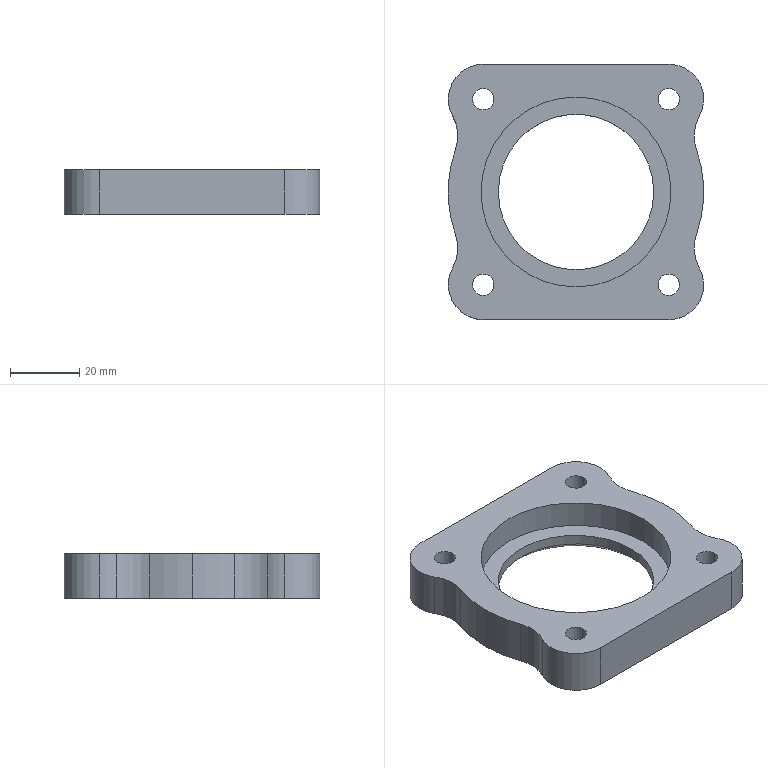Part | SolidWorks | features ICE 2, 3DProfileFeature 1, Chamfer 1, Extrusion 1, HoleWzd 1 | 1 solid | 34 faces | box 74 x 74 x 13 mm | volume 39480 mm3 | cylinder 27 | plane 5 | cone 2 | commonest cylinder face diameters 6.2 x8 20.2 x6 24 x6 74 x3 45 x2 55 x2
STEP:
#1=CARTESIAN_POINT('',(22.5,0.,2.));
#2=VERTEX_POINT('',#1);
#3=CARTESIAN_POINT('',(-22.5,0.,2.));
#4=VERTEX_POINT('',#3);
#5=CARTESIAN_POINT('',(0.,0.,2.));
#6=DIRECTION('',(0.,0.,-1.));
#7=DIRECTION('',(1.,0.,0.));
#8=AXIS2_PLACEMENT_3D('',#5,#6,#7);
#9=CIRCLE('',#8,22.5);
#10=EDGE_CURVE('',#2,#4,#9,.T.);
#11=ORIENTED_EDGE('',*,*,#10,.F.);
#12=CARTESIAN_POINT('',(24.5,0.,0.));
#13=VERTEX_POINT('',#12);
#14=CARTESIAN_POINT('',(22.5,0.,2.));
#15=DIRECTION('',(0.7071,0.,-0.7071));
#16=VECTOR('',#15,1000.);
#17=LINE('',#14,#16);
#18=EDGE_CURVE('',#2,#13,#17,.T.);
#19=ORIENTED_EDGE('',*,*,#18,.T.);
#20=CARTESIAN_POINT('',(-24.5,0.,0.));
#21=VERTEX_POINT('',#20);
#22=CARTESIAN_POINT('',(0.,0.,0.));
#23=DIRECTION('',(0.,0.,1.));
#24=DIRECTION('',(1.,0.,0.));
#25=AXIS2_PLACEMENT_3D('',#22,#23,#24);
#26=CIRCLE('',#25,24.5);
#27=EDGE_CURVE('',#21,#13,#26,.T.);
#28=ORIENTED_EDGE('',*,*,#27,.F.);
#29=CARTESIAN_POINT('',(-22.5,0.,2.));
#30=DIRECTION('',(-0.7071,0.,-0.7071));
#31=VECTOR('',#30,1000.);
#32=LINE('',#29,#31);
#33=EDGE_CURVE('',#4,#21,#32,.T.);
#34=ORIENTED_EDGE('',*,*,#33,.F.);
#35=EDGE_LOOP('',(#11,#19,#28,#34));
#36=FACE_OUTER_BOUND('',#35,.T.);
#37=CARTESIAN_POINT('',(0.,0.,2.));
#38=DIRECTION('',(0.,0.,-1.));
#39=DIRECTION('',(-1.,0.,0.));
#40=AXIS2_PLACEMENT_3D('',#37,#38,#39);
#41=CONICAL_SURFACE('',#40,22.5,0.7854);
#42=ADVANCED_FACE('',(#36),#41,.F.);
#43=ORIENTED_EDGE('',*,*,#10,.T.);
#44=CARTESIAN_POINT('',(-22.5,0.,5.));
#45=VERTEX_POINT('',#44);
#46=CARTESIAN_POINT('',(-22.5,0.,-0.001));
#47=DIRECTION('',(0.,0.,1.));
#48=VECTOR('',#47,1000.);
#49=LINE('',#46,#48);
#50=EDGE_CURVE('',#4,#45,#49,.T.);
#51=ORIENTED_EDGE('',*,*,#50,.T.);
#52=CARTESIAN_POINT('',(22.5,0.,5.));
#53=VERTEX_POINT('',#52);
#54=CARTESIAN_POINT('',(0.,0.,5.));
#55=DIRECTION('',(0.,0.,1.));
#56=DIRECTION('',(1.,0.,0.));
#57=AXIS2_PLACEMENT_3D('',#54,#55,#56);
#58=CIRCLE('',#57,22.5);
#59=EDGE_CURVE('',#45,#53,#58,.T.);
#60=ORIENTED_EDGE('',*,*,#59,.T.);
#61=CARTESIAN_POINT('',(22.5,0.,-0.001));
#62=DIRECTION('',(0.,0.,1.));
#63=VECTOR('',#62,1000.);
#64=LINE('',#61,#63);
#65=EDGE_CURVE('',#2,#53,#64,.T.);
#66=ORIENTED_EDGE('',*,*,#65,.F.);
#67=EDGE_LOOP('',(#43,#51,#60,#66));
#68=FACE_OUTER_BOUND('',#67,.T.);
#69=CARTESIAN_POINT('',(0.,0.,-0.001));
#70=DIRECTION('',(0.,0.,1.));
#71=DIRECTION('',(1.,0.,0.));
#72=AXIS2_PLACEMENT_3D('',#69,#70,#71);
#73=CYLINDRICAL_SURFACE('',#72,22.5);
#74=ADVANCED_FACE('',(#68),#73,.F.);
#75=CARTESIAN_POINT('',(-27.5,0.,5.));
#76=VERTEX_POINT('',#75);
#77=CARTESIAN_POINT('',(27.5,0.,5.));
#78=VERTEX_POINT('',#77);
#79=CARTESIAN_POINT('',(0.,0.,5.));
#80=DIRECTION('',(0.,0.,1.));
#81=DIRECTION('',(1.,0.,0.));
#82=AXIS2_PLACEMENT_3D('',#79,#80,#81);
#83=CIRCLE('',#82,27.5);
#84=EDGE_CURVE('',#76,#78,#83,.T.);
#85=ORIENTED_EDGE('',*,*,#84,.F.);
#86=CARTESIAN_POINT('',(-27.5,0.,13.));
#87=VERTEX_POINT('',#86);
#88=CARTESIAN_POINT('',(-27.5,0.,5.));
#89=DIRECTION('',(0.,0.,1.));
#90=VECTOR('',#89,1000.);
#91=LINE('',#88,#90);
#92=EDGE_CURVE('',#76,#87,#91,.T.);
#93=ORIENTED_EDGE('',*,*,#92,.T.);
#94=CARTESIAN_POINT('',(27.5,0.,13.));
#95=VERTEX_POINT('',#94);
#96=CARTESIAN_POINT('',(0.,0.,13.));
#97=DIRECTION('',(0.,0.,1.));
#98=DIRECTION('',(1.,0.,0.));
#99=AXIS2_PLACEMENT_3D('',#96,#97,#98);
#100=CIRCLE('',#99,27.5);
#101=EDGE_CURVE('',#87,#95,#100,.T.);
#102=ORIENTED_EDGE('',*,*,#101,.T.);
#103=CARTESIAN_POINT('',(27.5,0.,5.));
#104=DIRECTION('',(0.,0.,1.));
#105=VECTOR('',#104,1000.);
#106=LINE('',#103,#105);
#107=EDGE_CURVE('',#78,#95,#106,.T.);
#108=ORIENTED_EDGE('',*,*,#107,.F.);
#109=EDGE_LOOP('',(#85,#93,#102,#108));
#110=FACE_OUTER_BOUND('',#109,.T.);
#111=CARTESIAN_POINT('',(0.,0.,5.));
#112=DIRECTION('',(0.,0.,1.));
#113=DIRECTION('',(1.,0.,0.));
#114=AXIS2_PLACEMENT_3D('',#111,#112,#113);
#115=CYLINDRICAL_SURFACE('',#114,27.5);
#116=ADVANCED_FACE('',(#110),#115,.F.);
#117=CARTESIAN_POINT('',(-29.97,26.87,0.));
#118=VERTEX_POINT('',#117);
#119=CARTESIAN_POINT('',(-23.77,26.87,0.));
#120=VERTEX_POINT('',#119);
#121=CARTESIAN_POINT('',(-26.87,26.87,0.));
#122=DIRECTION('',(0.,0.,1.));
#123=DIRECTION('',(1.,0.,0.));
#124=AXIS2_PLACEMENT_3D('',#121,#122,#123);
#125=CIRCLE('',#124,3.1);
#126=EDGE_CURVE('',#118,#120,#125,.T.);
#127=ORIENTED_EDGE('',*,*,#126,.F.);
#128=CARTESIAN_POINT('',(-29.97,26.87,13.));
#129=VERTEX_POINT('',#128);
#130=CARTESIAN_POINT('',(-29.97,26.87,13.));
#131=DIRECTION('',(0.,0.,1.));
#132=VECTOR('',#131,1000.);
#133=LINE('',#130,#132);
#134=EDGE_CURVE('',#118,#129,#133,.T.);
#135=ORIENTED_EDGE('',*,*,#134,.T.);
#136=CARTESIAN_POINT('',(-23.77,26.87,13.));
#137=VERTEX_POINT('',#136);
#138=CARTESIAN_POINT('',(-26.87,26.87,13.));
#139=DIRECTION('',(0.,0.,1.));
#140=DIRECTION('',(1.,0.,0.));
#141=AXIS2_PLACEMENT_3D('',#138,#139,#140);
#142=CIRCLE('',#141,3.1);
#143=EDGE_CURVE('',#129,#137,#142,.T.);
#144=ORIENTED_EDGE('',*,*,#143,.T.);
#145=CARTESIAN_POINT('',(-23.77,26.87,13.));
#146=DIRECTION('',(0.,0.,1.));
#147=VECTOR('',#146,1000.);
#148=LINE('',#145,#147);
#149=EDGE_CURVE('',#120,#137,#148,.T.);
#150=ORIENTED_EDGE('',*,*,#149,.F.);
#151=EDGE_LOOP('',(#127,#135,#144,#150));
#152=FACE_OUTER_BOUND('',#151,.T.);
#153=CARTESIAN_POINT('',(-26.87,26.87,13.));
#154=DIRECTION('',(0.,0.,1.));
#155=DIRECTION('',(1.,0.,0.));
#156=AXIS2_PLACEMENT_3D('',#153,#154,#155);
#157=CYLINDRICAL_SURFACE('',#156,3.1);
#158=ADVANCED_FACE('',(#152),#157,.F.);
#159=CARTESIAN_POINT('',(23.77,26.87,0.));
#160=VERTEX_POINT('',#159);
#161=CARTESIAN_POINT('',(29.97,26.87,0.));
#162=VERTEX_POINT('',#161);
#163=CARTESIAN_POINT('',(26.87,26.87,0.));
#164=DIRECTION('',(0.,0.,1.));
#165=DIRECTION('',(1.,0.,0.));
#166=AXIS2_PLACEMENT_3D('',#163,#164,#165);
#167=CIRCLE('',#166,3.1);
#168=EDGE_CURVE('',#160,#162,#167,.T.);
#169=ORIENTED_EDGE('',*,*,#168,.F.);
#170=CARTESIAN_POINT('',(23.77,26.87,13.));
#171=VERTEX_POINT('',#170);
#172=CARTESIAN_POINT('',(23.77,26.87,13.));
#173=DIRECTION('',(0.,0.,1.));
#174=VECTOR('',#173,1000.);
#175=LINE('',#172,#174);
#176=EDGE_CURVE('',#160,#171,#175,.T.);
#177=ORIENTED_EDGE('',*,*,#176,.T.);
#178=CARTESIAN_POINT('',(29.97,26.87,13.));
#179=VERTEX_POINT('',#178);
#180=CARTESIAN_POINT('',(26.87,26.87,13.));
#181=DIRECTION('',(0.,0.,1.));
#182=DIRECTION('',(1.,0.,0.));
#183=AXIS2_PLACEMENT_3D('',#180,#181,#182);
#184=CIRCLE('',#183,3.1);
#185=EDGE_CURVE('',#171,#179,#184,.T.);
#186=ORIENTED_EDGE('',*,*,#185,.T.);
#187=CARTESIAN_POINT('',(29.97,26.87,13.));
#188=DIRECTION('',(0.,0.,1.));
#189=VECTOR('',#188,1000.);
#190=LINE('',#187,#189);
#191=EDGE_CURVE('',#162,#179,#190,.T.);
#192=ORIENTED_EDGE('',*,*,#191,.F.);
#193=EDGE_LOOP('',(#169,#177,#186,#192));
#194=FACE_OUTER_BOUND('',#193,.T.);
#195=CARTESIAN_POINT('',(26.87,26.87,13.));
#196=DIRECTION('',(0.,0.,1.));
#197=DIRECTION('',(1.,0.,0.));
#198=AXIS2_PLACEMENT_3D('',#195,#196,#197);
#199=CYLINDRICAL_SURFACE('',#198,3.1);
#200=ADVANCED_FACE('',(#194),#199,.F.);
#201=CARTESIAN_POINT('',(23.77,-26.87,0.));
#202=VERTEX_POINT('',#201);
#203=CARTESIAN_POINT('',(29.97,-26.87,0.));
#204=VERTEX_POINT('',#203);
#205=CARTESIAN_POINT('',(26.87,-26.87,0.));
#206=DIRECTION('',(0.,0.,1.));
#207=DIRECTION('',(1.,0.,0.));
#208=AXIS2_PLACEMENT_3D('',#205,#206,#207);
#209=CIRCLE('',#208,3.1);
#210=EDGE_CURVE('',#202,#204,#209,.T.);
#211=ORIENTED_EDGE('',*,*,#210,.F.);
#212=CARTESIAN_POINT('',(23.77,-26.87,13.));
#213=VERTEX_POINT('',#212);
#214=CARTESIAN_POINT('',(23.77,-26.87,13.));
#215=DIRECTION('',(0.,0.,1.));
#216=VECTOR('',#215,1000.);
#217=LINE('',#214,#216);
#218=EDGE_CURVE('',#202,#213,#217,.T.);
#219=ORIENTED_EDGE('',*,*,#218,.T.);
#220=CARTESIAN_POINT('',(29.97,-26.87,13.));
#221=VERTEX_POINT('',#220);
#222=CARTESIAN_POINT('',(26.87,-26.87,13.));
#223=DIRECTION('',(0.,0.,1.));
#224=DIRECTION('',(1.,0.,0.));
#225=AXIS2_PLACEMENT_3D('',#222,#223,#224);
#226=CIRCLE('',#225,3.1);
#227=EDGE_CURVE('',#213,#221,#226,.T.);
#228=ORIENTED_EDGE('',*,*,#227,.T.);
#229=CARTESIAN_POINT('',(29.97,-26.87,13.));
#230=DIRECTION('',(0.,0.,1.));
#231=VECTOR('',#230,1000.);
#232=LINE('',#229,#231);
#233=EDGE_CURVE('',#204,#221,#232,.T.);
#234=ORIENTED_EDGE('',*,*,#233,.F.);
#235=EDGE_LOOP('',(#211,#219,#228,#234));
#236=FACE_OUTER_BOUND('',#235,.T.);
#237=CARTESIAN_POINT('',(26.87,-26.87,13.));
#238=DIRECTION('',(0.,0.,1.));
#239=DIRECTION('',(1.,0.,0.));
#240=AXIS2_PLACEMENT_3D('',#237,#238,#239);
#241=CYLINDRICAL_SURFACE('',#240,3.1);
#242=ADVANCED_FACE('',(#236),#241,.F.);
#243=CARTESIAN_POINT('',(-29.97,-26.87,0.));
#244=VERTEX_POINT('',#243);
#245=CARTESIAN_POINT('',(-23.77,-26.87,0.));
#246=VERTEX_POINT('',#245);
#247=CARTESIAN_POINT('',(-26.87,-26.87,0.));
#248=DIRECTION('',(0.,0.,1.));
#249=DIRECTION('',(1.,0.,0.));
#250=AXIS2_PLACEMENT_3D('',#247,#248,#249);
#251=CIRCLE('',#250,3.1);
#252=EDGE_CURVE('',#244,#246,#251,.T.);
#253=ORIENTED_EDGE('',*,*,#252,.F.);
#254=CARTESIAN_POINT('',(-29.97,-26.87,13.));
#255=VERTEX_POINT('',#254);
#256=CARTESIAN_POINT('',(-29.97,-26.87,13.));
#257=DIRECTION('',(0.,0.,1.));
#258=VECTOR('',#257,1000.);
#259=LINE('',#256,#258);
#260=EDGE_CURVE('',#244,#255,#259,.T.);
#261=ORIENTED_EDGE('',*,*,#260,.T.);
#262=CARTESIAN_POINT('',(-23.77,-26.87,13.));
#263=VERTEX_POINT('',#262);
#264=CARTESIAN_POINT('',(-26.87,-26.87,13.));
#265=DIRECTION('',(0.,0.,1.));
#266=DIRECTION('',(1.,0.,0.));
#267=AXIS2_PLACEMENT_3D('',#264,#265,#266);
#268=CIRCLE('',#267,3.1);
#269=EDGE_CURVE('',#255,#263,#268,.T.);
#270=ORIENTED_EDGE('',*,*,#269,.T.);
#271=CARTESIAN_POINT('',(-23.77,-26.87,13.));
#272=DIRECTION('',(0.,0.,1.));
#273=VECTOR('',#272,1000.);
#274=LINE('',#271,#273);
#275=EDGE_CURVE('',#246,#263,#274,.T.);
#276=ORIENTED_EDGE('',*,*,#275,.F.);
#277=EDGE_LOOP('',(#253,#261,#270,#276));
#278=FACE_OUTER_BOUND('',#277,.T.);
#279=CARTESIAN_POINT('',(-26.87,-26.87,13.));
#280=DIRECTION('',(0.,0.,1.));
#281=DIRECTION('',(1.,0.,0.));
#282=AXIS2_PLACEMENT_3D('',#279,#280,#281);
#283=CYLINDRICAL_SURFACE('',#282,3.1);
#284=ADVANCED_FACE('',(#278),#283,.F.);
#285=CARTESIAN_POINT('',(-37.,0.,13.));
#286=VERTEX_POINT('',#285);
#287=CARTESIAN_POINT('',(-34.917,-12.239,13.));
#288=VERTEX_POINT('',#287);
#289=CARTESIAN_POINT('',(0.,0.,13.));
#290=DIRECTION('',(0.,0.,1.));
#291=DIRECTION('',(1.,0.,0.));
#292=AXIS2_PLACEMENT_3D('',#289,#290,#291);
#293=CIRCLE('',#292,37.);
#294=EDGE_CURVE('',#286,#288,#293,.T.);
#295=ORIENTED_EDGE('',*,*,#294,.F.);
#296=CARTESIAN_POINT('',(-37.,0.,0.));
#297=VERTEX_POINT('',#296);
#298=CARTESIAN_POINT('',(-37.,0.,13.));
#299=DIRECTION('',(0.,0.,-1.));
#300=VECTOR('',#299,1000.);
#301=LINE('',#298,#300);
#302=EDGE_CURVE('',#286,#297,#301,.T.);
#303=ORIENTED_EDGE('',*,*,#302,.T.);
#304=CARTESIAN_POINT('',(-34.917,-12.239,0.));
#305=VERTEX_POINT('',#304);
#306=CARTESIAN_POINT('',(0.,0.,0.));
#307=DIRECTION('',(0.,0.,1.));
#308=DIRECTION('',(1.,0.,0.));
#309=AXIS2_PLACEMENT_3D('',#306,#307,#308);
#310=CIRCLE('',#309,37.);
#311=EDGE_CURVE('',#297,#305,#310,.T.);
#312=ORIENTED_EDGE('',*,*,#311,.T.);
#313=CARTESIAN_POINT('',(-34.917,-12.239,13.));
#314=DIRECTION('',(0.,0.,-1.));
#315=VECTOR('',#314,1000.);
#316=LINE('',#313,#315);
#317=EDGE_CURVE('',#288,#305,#316,.T.);
#318=ORIENTED_EDGE('',*,*,#317,.F.);
#319=EDGE_LOOP('',(#295,#303,#312,#318));
#320=FACE_OUTER_BOUND('',#319,.T.);
#321=CARTESIAN_POINT('',(0.,0.,13.));
#322=DIRECTION('',(0.,0.,-1.));
#323=DIRECTION('',(-1.,0.,0.));
#324=AXIS2_PLACEMENT_3D('',#321,#322,#323);
#325=CYLINDRICAL_SURFACE('',#324,37.);
#326=ADVANCED_FACE('',(#320),#325,.T.);
#327=CARTESIAN_POINT('',(-35.739,22.014,13.));
#328=VERTEX_POINT('',#327);
#329=CARTESIAN_POINT('',(-37.,26.9,13.));
#330=VERTEX_POINT('',#329);
#331=CARTESIAN_POINT('',(-26.9,26.9,13.));
#332=DIRECTION('',(0.,0.,-1.));
#333=DIRECTION('',(1.,0.,0.));
#334=AXIS2_PLACEMENT_3D('',#331,#332,#333);
#335=CIRCLE('',#334,10.1);
#336=EDGE_CURVE('',#328,#330,#335,.T.);
#337=ORIENTED_EDGE('',*,*,#336,.T.);
#338=CARTESIAN_POINT('',(-37.,26.9,0.));
#339=VERTEX_POINT('',#338);
#340=CARTESIAN_POINT('',(-37.,26.9,13.));
#341=DIRECTION('',(0.,0.,-1.));
#342=VECTOR('',#341,1000.);
#343=LINE('',#340,#342);
#344=EDGE_CURVE('',#330,#339,#343,.T.);
#345=ORIENTED_EDGE('',*,*,#344,.T.);
#346=CARTESIAN_POINT('',(-35.739,22.014,0.));
#347=VERTEX_POINT('',#346);
#348=CARTESIAN_POINT('',(-26.9,26.9,0.));
#349=DIRECTION('',(0.,0.,-1.));
#350=DIRECTION('',(1.,0.,0.));
#351=AXIS2_PLACEMENT_3D('',#348,#349,#350);
#352=CIRCLE('',#351,10.1);
#353=EDGE_CURVE('',#347,#339,#352,.T.);
#354=ORIENTED_EDGE('',*,*,#353,.F.);
#355=CARTESIAN_POINT('',(-35.739,22.014,13.));
#356=DIRECTION('',(0.,0.,-1.));
#357=VECTOR('',#356,1000.);
#358=LINE('',#355,#357);
#359=EDGE_CURVE('',#328,#347,#358,.T.);
#360=ORIENTED_EDGE('',*,*,#359,.F.);
#361=EDGE_LOOP('',(#337,#345,#354,#360));
#362=FACE_OUTER_BOUND('',#361,.T.);
#363=CARTESIAN_POINT('',(-26.9,26.9,13.));
#364=DIRECTION('',(0.,0.,-1.));
#365=DIRECTION('',(-1.,0.,0.));
#366=AXIS2_PLACEMENT_3D('',#363,#364,#365);
#367=CYLINDRICAL_SURFACE('',#366,10.1);
#368=ADVANCED_FACE('',(#362),#367,.T.);
#369=CARTESIAN_POINT('',(34.242,16.208,13.));
#370=VERTEX_POINT('',#369);
#371=CARTESIAN_POINT('',(35.739,22.014,13.));
#372=VERTEX_POINT('',#371);
#373=CARTESIAN_POINT('',(46.242,16.208,13.));
#374=DIRECTION('',(0.,0.,-1.));
#375=DIRECTION('',(1.,0.,0.));
#376=AXIS2_PLACEMENT_3D('',#373,#374,#375);
#377=CIRCLE('',#376,12.);
#378=EDGE_CURVE('',#370,#372,#377,.T.);
#379=ORIENTED_EDGE('',*,*,#378,.F.);
#380=CARTESIAN_POINT('',(34.242,16.208,0.));
#381=VERTEX_POINT('',#380);
#382=CARTESIAN_POINT('',(34.242,16.208,13.));
#383=DIRECTION('',(0.,0.,-1.));
#384=VECTOR('',#383,1000.);
#385=LINE('',#382,#384);
#386=EDGE_CURVE('',#370,#381,#385,.T.);
#387=ORIENTED_EDGE('',*,*,#386,.T.);
#388=CARTESIAN_POINT('',(35.739,22.014,0.));
#389=VERTEX_POINT('',#388);
#390=CARTESIAN_POINT('',(46.242,16.208,0.));
#391=DIRECTION('',(0.,0.,-1.));
#392=DIRECTION('',(1.,0.,0.));
#393=AXIS2_PLACEMENT_3D('',#390,#391,#392);
#394=CIRCLE('',#393,12.);
#395=EDGE_CURVE('',#381,#389,#394,.T.);
#396=ORIENTED_EDGE('',*,*,#395,.T.);
#397=CARTESIAN_POINT('',(35.739,22.014,13.));
#398=DIRECTION('',(0.,0.,-1.));
#399=VECTOR('',#398,1000.);
#400=LINE('',#397,#399);
#401=EDGE_CURVE('',#372,#389,#400,.T.);
#402=ORIENTED_EDGE('',*,*,#401,.F.);
#403=EDGE_LOOP('',(#379,#387,#396,#402));
#404=FACE_OUTER_BOUND('',#403,.T.);
#405=CARTESIAN_POINT('',(46.242,16.208,13.));
#406=DIRECTION('',(0.,0.,-1.));
#407=DIRECTION('',(-1.,0.,0.));
#408=AXIS2_PLACEMENT_3D('',#405,#406,#407);
#409=CYLINDRICAL_SURFACE('',#408,12.);
#410=ADVANCED_FACE('',(#404),#409,.F.);
#411=CARTESIAN_POINT('',(34.917,-12.239,13.));
#412=VERTEX_POINT('',#411);
#413=CARTESIAN_POINT('',(34.242,-16.208,13.));
#414=VERTEX_POINT('',#413);
#415=CARTESIAN_POINT('',(46.242,-16.208,13.));
#416=DIRECTION('',(0.,0.,1.));
#417=DIRECTION('',(1.,0.,0.));
#418=AXIS2_PLACEMENT_3D('',#415,#416,#417);
#419=CIRCLE('',#418,12.);
#420=EDGE_CURVE('',#412,#414,#419,.T.);
#421=ORIENTED_EDGE('',*,*,#420,.T.);
#422=CARTESIAN_POINT('',(34.242,-16.208,0.));
#423=VERTEX_POINT('',#422);
#424=CARTESIAN_POINT('',(34.242,-16.208,13.));
#425=DIRECTION('',(0.,0.,-1.));
#426=VECTOR('',#425,1000.);
#427=LINE('',#424,#426);
#428=EDGE_CURVE('',#414,#423,#427,.T.);
#429=ORIENTED_EDGE('',*,*,#428,.T.);
#430=CARTESIAN_POINT('',(34.917,-12.239,0.));
#431=VERTEX_POINT('',#430);
#432=CARTESIAN_POINT('',(46.242,-16.208,0.));
#433=DIRECTION('',(0.,0.,1.));
#434=DIRECTION('',(1.,0.,0.));
#435=AXIS2_PLACEMENT_3D('',#432,#433,#434);
#436=CIRCLE('',#435,12.);
#437=EDGE_CURVE('',#431,#423,#436,.T.);
#438=ORIENTED_EDGE('',*,*,#437,.F.);
#439=CARTESIAN_POINT('',(34.917,-12.239,13.));
#440=DIRECTION('',(0.,0.,-1.));
#441=VECTOR('',#440,1000.);
#442=LINE('',#439,#441);
#443=EDGE_CURVE('',#412,#431,#442,.T.);
#444=ORIENTED_EDGE('',*,*,#443,.F.);
#445=EDGE_LOOP('',(#421,#429,#438,#444));
#446=FACE_OUTER_BOUND('',#445,.T.);
#447=CARTESIAN_POINT('',(46.242,-16.208,13.));
#448=DIRECTION('',(0.,0.,-1.));
#449=DIRECTION('',(-1.,0.,0.));
#450=AXIS2_PLACEMENT_3D('',#447,#448,#449);
#451=CYLINDRICAL_SURFACE('',#450,12.);
#452=ADVANCED_FACE('',(#446),#451,.F.);
#453=CARTESIAN_POINT('',(-37.,-26.9,13.));
#454=VERTEX_POINT('',#453);
#455=CARTESIAN_POINT('',(-26.9,-37.,13.));
#456=VERTEX_POINT('',#455);
#457=CARTESIAN_POINT('',(-26.9,-26.9,13.));
#458=DIRECTION('',(0.,0.,1.));
#459=DIRECTION('',(1.,0.,0.));
#460=AXIS2_PLACEMENT_3D('',#457,#458,#459);
#461=CIRCLE('',#460,10.1);
#462=EDGE_CURVE('',#454,#456,#461,.T.);
#463=ORIENTED_EDGE('',*,*,#462,.F.);
#464=CARTESIAN_POINT('',(-37.,-26.9,0.));
#465=VERTEX_POINT('',#464);
#466=CARTESIAN_POINT('',(-37.,-26.9,13.));
#467=DIRECTION('',(0.,0.,-1.));
#468=VECTOR('',#467,1000.);
#469=LINE('',#466,#468);
#470=EDGE_CURVE('',#454,#465,#469,.T.);
#471=ORIENTED_EDGE('',*,*,#470,.T.);
#472=CARTESIAN_POINT('',(-26.9,-37.,0.));
#473=VERTEX_POINT('',#472);
#474=CARTESIAN_POINT('',(-26.9,-26.9,0.));
#475=DIRECTION('',(0.,0.,1.));
#476=DIRECTION('',(1.,0.,0.));
#477=AXIS2_PLACEMENT_3D('',#474,#475,#476);
#478=CIRCLE('',#477,10.1);
#479=EDGE_CURVE('',#465,#473,#478,.T.);
#480=ORIENTED_EDGE('',*,*,#479,.T.);
#481=CARTESIAN_POINT('',(-26.9,-37.,13.));
#482=DIRECTION('',(0.,0.,-1.));
#483=VECTOR('',#482,1000.);
#484=LINE('',#481,#483);
#485=EDGE_CURVE('',#456,#473,#484,.T.);
#486=ORIENTED_EDGE('',*,*,#485,.F.);
#487=EDGE_LOOP('',(#463,#471,#480,#486));
#488=FACE_OUTER_BOUND('',#487,.T.);
#489=CARTESIAN_POINT('',(-26.9,-26.9,13.));
#490=DIRECTION('',(0.,0.,-1.));
#491=DIRECTION('',(-1.,0.,0.));
#492=AXIS2_PLACEMENT_3D('',#489,#490,#491);
#493=CYLINDRICAL_SURFACE('',#492,10.1);
#494=ADVANCED_FACE('',(#488),#493,.T.);
#495=CARTESIAN_POINT('',(-35.739,-22.014,0.));
#496=VERTEX_POINT('',#495);
#497=CARTESIAN_POINT('',(-46.242,-16.208,0.));
#498=DIRECTION('',(0.,0.,-1.));
#499=DIRECTION('',(1.,0.,0.));
#500=AXIS2_PLACEMENT_3D('',#497,#498,#499);
#501=CIRCLE('',#500,12.);
#502=EDGE_CURVE('',#305,#496,#501,.T.);
#503=ORIENTED_EDGE('',*,*,#502,.T.);
#504=CARTESIAN_POINT('',(-35.739,-22.014,13.));
#505=VERTEX_POINT('',#504);
#506=CARTESIAN_POINT('',(-35.739,-22.014,13.));
#507=DIRECTION('',(0.,0.,-1.));
#508=VECTOR('',#507,1000.);
#509=LINE('',#506,#508);
#510=EDGE_CURVE('',#505,#496,#509,.T.);
#511=ORIENTED_EDGE('',*,*,#510,.F.);
#512=CARTESIAN_POINT('',(-46.242,-16.208,13.));
#513=DIRECTION('',(0.,0.,-1.));
#514=DIRECTION('',(1.,0.,0.));
#515=AXIS2_PLACEMENT_3D('',#512,#513,#514);
#516=CIRCLE('',#515,12.);
#517=EDGE_CURVE('',#288,#505,#516,.T.);
#518=ORIENTED_EDGE('',*,*,#517,.F.);
#519=ORIENTED_EDGE('',*,*,#317,.T.);
#520=EDGE_LOOP('',(#503,#511,#518,#519));
#521=FACE_OUTER_BOUND('',#520,.T.);
#522=CARTESIAN_POINT('',(-46.242,-16.208,13.));
#523=DIRECTION('',(0.,0.,-1.));
#524=DIRECTION('',(-1.,0.,0.));
#525=AXIS2_PLACEMENT_3D('',#522,#523,#524);
#526=CYLINDRICAL_SURFACE('',#525,12.);
#527=ADVANCED_FACE('',(#521),#526,.F.);
#528=ORIENTED_EDGE('',*,*,#470,.F.);
#529=CARTESIAN_POINT('',(-26.9,-26.9,13.));
#530=DIRECTION('',(0.,0.,1.));
#531=DIRECTION('',(1.,0.,0.));
#532=AXIS2_PLACEMENT_3D('',#529,#530,#531);
#533=CIRCLE('',#532,10.1);
#534=EDGE_CURVE('',#505,#454,#533,.T.);
#535=ORIENTED_EDGE('',*,*,#534,.F.);
#536=ORIENTED_EDGE('',*,*,#510,.T.);
#537=CARTESIAN_POINT('',(-26.9,-26.9,0.));
#538=DIRECTION('',(0.,0.,1.));
#539=DIRECTION('',(1.,0.,0.));
#540=AXIS2_PLACEMENT_3D('',#537,#538,#539);
#541=CIRCLE('',#540,10.1);
#542=EDGE_CURVE('',#496,#465,#541,.T.);
#543=ORIENTED_EDGE('',*,*,#542,.T.);
#544=EDGE_LOOP('',(#528,#535,#536,#543));
#545=FACE_OUTER_BOUND('',#544,.T.);
#546=CARTESIAN_POINT('',(-26.9,-26.9,13.));
#547=DIRECTION('',(0.,0.,-1.));
#548=DIRECTION('',(-1.,0.,0.));
#549=AXIS2_PLACEMENT_3D('',#546,#547,#548);
#550=CYLINDRICAL_SURFACE('',#549,10.1);
#551=ADVANCED_FACE('',(#545),#550,.T.);
#552=CARTESIAN_POINT('',(26.9,-37.,0.));
#553=VERTEX_POINT('',#552);
#554=CARTESIAN_POINT('',(0.,-37.,0.));
#555=DIRECTION('',(1.,0.,0.));
#556=VECTOR('',#555,1000.);
#557=LINE('',#554,#556);
#558=EDGE_CURVE('',#473,#553,#557,.T.);
#559=ORIENTED_EDGE('',*,*,#558,.T.);
#560=CARTESIAN_POINT('',(26.9,-37.,13.));
#561=VERTEX_POINT('',#560);
#562=CARTESIAN_POINT('',(26.9,-37.,13.));
#563=DIRECTION('',(0.,0.,-1.));
#564=VECTOR('',#563,1000.);
#565=LINE('',#562,#564);
#566=EDGE_CURVE('',#561,#553,#565,.T.);
#567=ORIENTED_EDGE('',*,*,#566,.F.);
#568=CARTESIAN_POINT('',(0.,-37.,13.));
#569=DIRECTION('',(1.,0.,0.));
#570=VECTOR('',#569,1000.);
#571=LINE('',#568,#570);
#572=EDGE_CURVE('',#456,#561,#571,.T.);
#573=ORIENTED_EDGE('',*,*,#572,.F.);
#574=ORIENTED_EDGE('',*,*,#485,.T.);
#575=EDGE_LOOP('',(#559,#567,#573,#574));
#576=FACE_OUTER_BOUND('',#575,.T.);
#577=CARTESIAN_POINT('',(0.,-37.,13.));
#578=DIRECTION('',(0.,1.,0.));
#579=DIRECTION('',(0.,0.,1.));
#580=AXIS2_PLACEMENT_3D('',#577,#578,#579);
#581=PLANE('',#580);
#582=ADVANCED_FACE('',(#576),#581,.F.);
#583=CARTESIAN_POINT('',(35.739,-22.014,0.));
#584=VERTEX_POINT('',#583);
#585=CARTESIAN_POINT('',(26.9,-26.9,0.));
#586=DIRECTION('',(0.,0.,-1.));
#587=DIRECTION('',(1.,0.,0.));
#588=AXIS2_PLACEMENT_3D('',#585,#586,#587);
#589=CIRCLE('',#588,10.1);
#590=EDGE_CURVE('',#584,#553,#589,.T.);
#591=ORIENTED_EDGE('',*,*,#590,.F.);
#592=CARTESIAN_POINT('',(35.739,-22.014,13.));
#593=VERTEX_POINT('',#592);
#594=CARTESIAN_POINT('',(35.739,-22.014,13.));
#595=DIRECTION('',(0.,0.,-1.));
#596=VECTOR('',#595,1000.);
#597=LINE('',#594,#596);
#598=EDGE_CURVE('',#593,#584,#597,.T.);
#599=ORIENTED_EDGE('',*,*,#598,.F.);
#600=CARTESIAN_POINT('',(26.9,-26.9,13.));
#601=DIRECTION('',(0.,0.,-1.));
#602=DIRECTION('',(1.,0.,0.));
#603=AXIS2_PLACEMENT_3D('',#600,#601,#602);
#604=CIRCLE('',#603,10.1);
#605=EDGE_CURVE('',#593,#561,#604,.T.);
#606=ORIENTED_EDGE('',*,*,#605,.T.);
#607=ORIENTED_EDGE('',*,*,#566,.T.);
#608=EDGE_LOOP('',(#591,#599,#606,#607));
#609=FACE_OUTER_BOUND('',#608,.T.);
#610=CARTESIAN_POINT('',(26.9,-26.9,13.));
#611=DIRECTION('',(0.,0.,-1.));
#612=DIRECTION('',(-1.,0.,0.));
#613=AXIS2_PLACEMENT_3D('',#610,#611,#612);
#614=CYLINDRICAL_SURFACE('',#613,10.1);
#615=ADVANCED_FACE('',(#609),#614,.T.);
#616=ORIENTED_EDGE('',*,*,#428,.F.);
#617=CARTESIAN_POINT('',(46.242,-16.208,13.));
#618=DIRECTION('',(0.,0.,1.));
#619=DIRECTION('',(1.,0.,0.));
#620=AXIS2_PLACEMENT_3D('',#617,#618,#619);
#621=CIRCLE('',#620,12.);
#622=EDGE_CURVE('',#414,#593,#621,.T.);
#623=ORIENTED_EDGE('',*,*,#622,.T.);
#624=ORIENTED_EDGE('',*,*,#598,.T.);
#625=CARTESIAN_POINT('',(46.242,-16.208,0.));
#626=DIRECTION('',(0.,0.,1.));
#627=DIRECTION('',(1.,0.,0.));
#628=AXIS2_PLACEMENT_3D('',#625,#626,#627);
#629=CIRCLE('',#628,12.);
#630=EDGE_CURVE('',#423,#584,#629,.T.);
#631=ORIENTED_EDGE('',*,*,#630,.F.);
#632=EDGE_LOOP('',(#616,#623,#624,#631));
#633=FACE_OUTER_BOUND('',#632,.T.);
#634=CARTESIAN_POINT('',(46.242,-16.208,13.));
#635=DIRECTION('',(0.,0.,-1.));
#636=DIRECTION('',(-1.,0.,0.));
#637=AXIS2_PLACEMENT_3D('',#634,#635,#636);
#638=CYLINDRICAL_SURFACE('',#637,12.);
#639=ADVANCED_FACE('',(#633),#638,.F.);
#640=CARTESIAN_POINT('',(34.917,12.239,0.));
#641=VERTEX_POINT('',#640);
#642=CARTESIAN_POINT('',(0.,0.,0.));
#643=DIRECTION('',(0.,0.,-1.));
#644=DIRECTION('',(1.,0.,0.));
#645=AXIS2_PLACEMENT_3D('',#642,#643,#644);
#646=CIRCLE('',#645,37.);
#647=EDGE_CURVE('',#641,#431,#646,.T.);
#648=ORIENTED_EDGE('',*,*,#647,.F.);
#649=CARTESIAN_POINT('',(34.917,12.239,13.));
#650=VERTEX_POINT('',#649);
#651=CARTESIAN_POINT('',(34.917,12.239,13.));
#652=DIRECTION('',(0.,0.,-1.));
#653=VECTOR('',#652,1000.);
#654=LINE('',#651,#653);
#655=EDGE_CURVE('',#650,#641,#654,.T.);
#656=ORIENTED_EDGE('',*,*,#655,.F.);
#657=CARTESIAN_POINT('',(0.,0.,13.));
#658=DIRECTION('',(0.,0.,-1.));
#659=DIRECTION('',(1.,0.,0.));
#660=AXIS2_PLACEMENT_3D('',#657,#658,#659);
#661=CIRCLE('',#660,37.);
#662=EDGE_CURVE('',#650,#412,#661,.T.);
#663=ORIENTED_EDGE('',*,*,#662,.T.);
#664=ORIENTED_EDGE('',*,*,#443,.T.);
#665=EDGE_LOOP('',(#648,#656,#663,#664));
#666=FACE_OUTER_BOUND('',#665,.T.);
#667=CARTESIAN_POINT('',(0.,0.,13.));
#668=DIRECTION('',(0.,0.,-1.));
#669=DIRECTION('',(-1.,0.,0.));
#670=AXIS2_PLACEMENT_3D('',#667,#668,#669);
#671=CYLINDRICAL_SURFACE('',#670,37.);
#672=ADVANCED_FACE('',(#666),#671,.T.);
#673=ORIENTED_EDGE('',*,*,#386,.F.);
#674=CARTESIAN_POINT('',(46.242,16.208,13.));
#675=DIRECTION('',(0.,0.,-1.));
#676=DIRECTION('',(1.,0.,0.));
#677=AXIS2_PLACEMENT_3D('',#674,#675,#676);
#678=CIRCLE('',#677,12.);
#679=EDGE_CURVE('',#650,#370,#678,.T.);
#680=ORIENTED_EDGE('',*,*,#679,.F.);
#681=ORIENTED_EDGE('',*,*,#655,.T.);
#682=CARTESIAN_POINT('',(46.242,16.208,0.));
#683=DIRECTION('',(0.,0.,-1.));
#684=DIRECTION('',(1.,0.,0.));
#685=AXIS2_PLACEMENT_3D('',#682,#683,#684);
#686=CIRCLE('',#685,12.);
#687=EDGE_CURVE('',#641,#381,#686,.T.);
#688=ORIENTED_EDGE('',*,*,#687,.T.);
#689=EDGE_LOOP('',(#673,#680,#681,#688));
#690=FACE_OUTER_BOUND('',#689,.T.);
#691=CARTESIAN_POINT('',(46.242,16.208,13.));
#692=DIRECTION('',(0.,0.,-1.));
#693=DIRECTION('',(-1.,0.,0.));
#694=AXIS2_PLACEMENT_3D('',#691,#692,#693);
#695=CYLINDRICAL_SURFACE('',#694,12.);
#696=ADVANCED_FACE('',(#690),#695,.F.);
#697=CARTESIAN_POINT('',(26.9,37.,0.));
#698=VERTEX_POINT('',#697);
#699=CARTESIAN_POINT('',(26.9,26.9,0.));
#700=DIRECTION('',(0.,0.,1.));
#701=DIRECTION('',(1.,0.,0.));
#702=AXIS2_PLACEMENT_3D('',#699,#700,#701);
#703=CIRCLE('',#702,10.1);
#704=EDGE_CURVE('',#389,#698,#703,.T.);
#705=ORIENTED_EDGE('',*,*,#704,.T.);
#706=CARTESIAN_POINT('',(26.9,37.,13.));
#707=VERTEX_POINT('',#706);
#708=CARTESIAN_POINT('',(26.9,37.,13.));
#709=DIRECTION('',(0.,0.,-1.));
#710=VECTOR('',#709,1000.);
#711=LINE('',#708,#710);
#712=EDGE_CURVE('',#707,#698,#711,.T.);
#713=ORIENTED_EDGE('',*,*,#712,.F.);
#714=CARTESIAN_POINT('',(26.9,26.9,13.));
#715=DIRECTION('',(0.,0.,1.));
#716=DIRECTION('',(1.,0.,0.));
#717=AXIS2_PLACEMENT_3D('',#714,#715,#716);
#718=CIRCLE('',#717,10.1);
#719=EDGE_CURVE('',#372,#707,#718,.T.);
#720=ORIENTED_EDGE('',*,*,#719,.F.);
#721=ORIENTED_EDGE('',*,*,#401,.T.);
#722=EDGE_LOOP('',(#705,#713,#720,#721));
#723=FACE_OUTER_BOUND('',#722,.T.);
#724=CARTESIAN_POINT('',(26.9,26.9,13.));
#725=DIRECTION('',(0.,0.,-1.));
#726=DIRECTION('',(-1.,0.,0.));
#727=AXIS2_PLACEMENT_3D('',#724,#725,#726);
#728=CYLINDRICAL_SURFACE('',#727,10.1);
#729=ADVANCED_FACE('',(#723),#728,.T.);
#730=CARTESIAN_POINT('',(-26.9,37.,0.));
#731=VERTEX_POINT('',#730);
#732=CARTESIAN_POINT('',(0.,37.,0.));
#733=DIRECTION('',(1.,0.,0.));
#734=VECTOR('',#733,1000.);
#735=LINE('',#732,#734);
#736=EDGE_CURVE('',#731,#698,#735,.T.);
#737=ORIENTED_EDGE('',*,*,#736,.F.);
#738=CARTESIAN_POINT('',(-26.9,37.,13.));
#739=VERTEX_POINT('',#738);
#740=CARTESIAN_POINT('',(-26.9,37.,13.));
#741=DIRECTION('',(0.,0.,-1.));
#742=VECTOR('',#741,1000.);
#743=LINE('',#740,#742);
#744=EDGE_CURVE('',#739,#731,#743,.T.);
#745=ORIENTED_EDGE('',*,*,#744,.F.);
#746=CARTESIAN_POINT('',(0.,37.,13.));
#747=DIRECTION('',(1.,0.,0.));
#748=VECTOR('',#747,1000.);
#749=LINE('',#746,#748);
#750=EDGE_CURVE('',#739,#707,#749,.T.);
#751=ORIENTED_EDGE('',*,*,#750,.T.);
#752=ORIENTED_EDGE('',*,*,#712,.T.);
#753=EDGE_LOOP('',(#737,#745,#751,#752));
#754=FACE_OUTER_BOUND('',#753,.T.);
#755=CARTESIAN_POINT('',(0.,37.,13.));
#756=DIRECTION('',(0.,1.,0.));
#757=DIRECTION('',(0.,0.,1.));
#758=AXIS2_PLACEMENT_3D('',#755,#756,#757);
#759=PLANE('',#758);
#760=ADVANCED_FACE('',(#754),#759,.T.);
#761=ORIENTED_EDGE('',*,*,#344,.F.);
#762=CARTESIAN_POINT('',(-26.9,26.9,13.));
#763=DIRECTION('',(0.,0.,-1.));
#764=DIRECTION('',(1.,0.,0.));
#765=AXIS2_PLACEMENT_3D('',#762,#763,#764);
#766=CIRCLE('',#765,10.1);
#767=EDGE_CURVE('',#330,#739,#766,.T.);
#768=ORIENTED_EDGE('',*,*,#767,.T.);
#769=ORIENTED_EDGE('',*,*,#744,.T.);
#770=CARTESIAN_POINT('',(-26.9,26.9,0.));
#771=DIRECTION('',(0.,0.,-1.));
#772=DIRECTION('',(1.,0.,0.));
#773=AXIS2_PLACEMENT_3D('',#770,#771,#772);
#774=CIRCLE('',#773,10.1);
#775=EDGE_CURVE('',#339,#731,#774,.T.);
#776=ORIENTED_EDGE('',*,*,#775,.F.);
#777=EDGE_LOOP('',(#761,#768,#769,#776));
#778=FACE_OUTER_BOUND('',#777,.T.);
#779=CARTESIAN_POINT('',(-26.9,26.9,13.));
#780=DIRECTION('',(0.,0.,-1.));
#781=DIRECTION('',(-1.,0.,0.));
#782=AXIS2_PLACEMENT_3D('',#779,#780,#781);
#783=CYLINDRICAL_SURFACE('',#782,10.1);
#784=ADVANCED_FACE('',(#778),#783,.T.);
#785=CARTESIAN_POINT('',(-34.917,12.239,0.));
#786=VERTEX_POINT('',#785);
#787=CARTESIAN_POINT('',(-46.242,16.208,0.));
#788=DIRECTION('',(0.,0.,1.));
#789=DIRECTION('',(1.,0.,0.));
#790=AXIS2_PLACEMENT_3D('',#787,#788,#789);
#791=CIRCLE('',#790,12.);
#792=EDGE_CURVE('',#786,#347,#791,.T.);
#793=ORIENTED_EDGE('',*,*,#792,.F.);
#794=CARTESIAN_POINT('',(-34.917,12.239,13.));
#795=VERTEX_POINT('',#794);
#796=CARTESIAN_POINT('',(-34.917,12.239,13.));
#797=DIRECTION('',(0.,0.,-1.));
#798=VECTOR('',#797,1000.);
#799=LINE('',#796,#798);
#800=EDGE_CURVE('',#795,#786,#799,.T.);
#801=ORIENTED_EDGE('',*,*,#800,.F.);
#802=CARTESIAN_POINT('',(-46.242,16.208,13.));
#803=DIRECTION('',(0.,0.,1.));
#804=DIRECTION('',(1.,0.,0.));
#805=AXIS2_PLACEMENT_3D('',#802,#803,#804);
#806=CIRCLE('',#805,12.);
#807=EDGE_CURVE('',#795,#328,#806,.T.);
#808=ORIENTED_EDGE('',*,*,#807,.T.);
#809=ORIENTED_EDGE('',*,*,#359,.T.);
#810=EDGE_LOOP('',(#793,#801,#808,#809));
#811=FACE_OUTER_BOUND('',#810,.T.);
#812=CARTESIAN_POINT('',(-46.242,16.208,13.));
#813=DIRECTION('',(0.,0.,-1.));
#814=DIRECTION('',(-1.,0.,0.));
#815=AXIS2_PLACEMENT_3D('',#812,#813,#814);
#816=CYLINDRICAL_SURFACE('',#815,12.);
#817=ADVANCED_FACE('',(#811),#816,.F.);
#818=ORIENTED_EDGE('',*,*,#302,.F.);
#819=CARTESIAN_POINT('',(0.,0.,13.));
#820=DIRECTION('',(0.,0.,1.));
#821=DIRECTION('',(1.,0.,0.));
#822=AXIS2_PLACEMENT_3D('',#819,#820,#821);
#823=CIRCLE('',#822,37.);
#824=EDGE_CURVE('',#795,#286,#823,.T.);
#825=ORIENTED_EDGE('',*,*,#824,.F.);
#826=ORIENTED_EDGE('',*,*,#800,.T.);
#827=CARTESIAN_POINT('',(0.,0.,0.));
#828=DIRECTION('',(0.,0.,1.));
#829=DIRECTION('',(1.,0.,0.));
#830=AXIS2_PLACEMENT_3D('',#827,#828,#829);
#831=CIRCLE('',#830,37.);
#832=EDGE_CURVE('',#786,#297,#831,.T.);
#833=ORIENTED_EDGE('',*,*,#832,.T.);
#834=EDGE_LOOP('',(#818,#825,#826,#833));
#835=FACE_OUTER_BOUND('',#834,.T.);
#836=CARTESIAN_POINT('',(0.,0.,13.));
#837=DIRECTION('',(0.,0.,-1.));
#838=DIRECTION('',(-1.,0.,0.));
#839=AXIS2_PLACEMENT_3D('',#836,#837,#838);
#840=CYLINDRICAL_SURFACE('',#839,37.);
#841=ADVANCED_FACE('',(#835),#840,.T.);
#842=CARTESIAN_POINT('',(0.,0.,13.));
#843=DIRECTION('',(0.,0.,1.));
#844=DIRECTION('',(1.,0.,0.));
#845=AXIS2_PLACEMENT_3D('',#842,#843,#844);
#846=CIRCLE('',#845,27.5);
#847=EDGE_CURVE('',#95,#87,#846,.T.);
#848=ORIENTED_EDGE('',*,*,#847,.F.);
#849=ORIENTED_EDGE('',*,*,#101,.F.);
#850=EDGE_LOOP('',(#848,#849));
#851=FACE_BOUND('',#850,.T.);
#852=CARTESIAN_POINT('',(-26.87,26.87,13.));
#853=DIRECTION('',(0.,0.,1.));
#854=DIRECTION('',(1.,0.,0.));
#855=AXIS2_PLACEMENT_3D('',#852,#853,#854);
#856=CIRCLE('',#855,3.1);
#857=EDGE_CURVE('',#137,#129,#856,.T.);
#858=ORIENTED_EDGE('',*,*,#857,.F.);
#859=ORIENTED_EDGE('',*,*,#143,.F.);
#860=EDGE_LOOP('',(#858,#859));
#861=FACE_BOUND('',#860,.T.);
#862=CARTESIAN_POINT('',(26.87,26.87,13.));
#863=DIRECTION('',(0.,0.,1.));
#864=DIRECTION('',(1.,0.,0.));
#865=AXIS2_PLACEMENT_3D('',#862,#863,#864);
#866=CIRCLE('',#865,3.1);
#867=EDGE_CURVE('',#179,#171,#866,.T.);
#868=ORIENTED_EDGE('',*,*,#867,.F.);
#869=ORIENTED_EDGE('',*,*,#185,.F.);
#870=EDGE_LOOP('',(#868,#869));
#871=FACE_BOUND('',#870,.T.);
#872=CARTESIAN_POINT('',(26.87,-26.87,13.));
#873=DIRECTION('',(0.,0.,1.));
#874=DIRECTION('',(1.,0.,0.));
#875=AXIS2_PLACEMENT_3D('',#872,#873,#874);
#876=CIRCLE('',#875,3.1);
#877=EDGE_CURVE('',#221,#213,#876,.T.);
#878=ORIENTED_EDGE('',*,*,#877,.F.);
#879=ORIENTED_EDGE('',*,*,#227,.F.);
#880=EDGE_LOOP('',(#878,#879));
#881=FACE_BOUND('',#880,.T.);
#882=CARTESIAN_POINT('',(-26.87,-26.87,13.));
#883=DIRECTION('',(0.,0.,1.));
#884=DIRECTION('',(1.,0.,0.));
#885=AXIS2_PLACEMENT_3D('',#882,#883,#884);
#886=CIRCLE('',#885,3.1);
#887=EDGE_CURVE('',#263,#255,#886,.T.);
#888=ORIENTED_EDGE('',*,*,#887,.F.);
#889=ORIENTED_EDGE('',*,*,#269,.F.);
#890=EDGE_LOOP('',(#888,#889));
#891=FACE_BOUND('',#890,.T.);
#892=ORIENTED_EDGE('',*,*,#517,.T.);
#893=ORIENTED_EDGE('',*,*,#534,.T.);
#894=ORIENTED_EDGE('',*,*,#462,.T.);
#895=ORIENTED_EDGE('',*,*,#572,.T.);
#896=ORIENTED_EDGE('',*,*,#605,.F.);
#897=ORIENTED_EDGE('',*,*,#622,.F.);
#898=ORIENTED_EDGE('',*,*,#420,.F.);
#899=ORIENTED_EDGE('',*,*,#662,.F.);
#900=ORIENTED_EDGE('',*,*,#679,.T.);
#901=ORIENTED_EDGE('',*,*,#378,.T.);
#902=ORIENTED_EDGE('',*,*,#719,.T.);
#903=ORIENTED_EDGE('',*,*,#750,.F.);
#904=ORIENTED_EDGE('',*,*,#767,.F.);
#905=ORIENTED_EDGE('',*,*,#336,.F.);
#906=ORIENTED_EDGE('',*,*,#807,.F.);
#907=ORIENTED_EDGE('',*,*,#824,.T.);
#908=ORIENTED_EDGE('',*,*,#294,.T.);
#909=EDGE_LOOP('',(#892,#893,#894,#895,#896,#897,#898,#899,#900,#901,#902,#903,#904,#905,#906,#907,#908));
#910=FACE_OUTER_BOUND('',#909,.T.);
#911=CARTESIAN_POINT('',(0.,0.,13.));
#912=DIRECTION('',(0.,0.,1.));
#913=DIRECTION('',(1.,0.,0.));
#914=AXIS2_PLACEMENT_3D('',#911,#912,#913);
#915=PLANE('',#914);
#916=ADVANCED_FACE('',(#851,#861,#871,#881,#891,#910),#915,.T.);
#917=ORIENTED_EDGE('',*,*,#27,.T.);
#918=CARTESIAN_POINT('',(0.,0.,0.));
#919=DIRECTION('',(0.,0.,1.));
#920=DIRECTION('',(1.,0.,0.));
#921=AXIS2_PLACEMENT_3D('',#918,#919,#920);
#922=CIRCLE('',#921,24.5);
#923=EDGE_CURVE('',#13,#21,#922,.T.);
#924=ORIENTED_EDGE('',*,*,#923,.T.);
#925=EDGE_LOOP('',(#917,#924));
#926=FACE_BOUND('',#925,.T.);
#927=CARTESIAN_POINT('',(-26.87,26.87,0.));
#928=DIRECTION('',(0.,0.,1.));
#929=DIRECTION('',(1.,0.,0.));
#930=AXIS2_PLACEMENT_3D('',#927,#928,#929);
#931=CIRCLE('',#930,3.1);
#932=EDGE_CURVE('',#120,#118,#931,.T.);
#933=ORIENTED_EDGE('',*,*,#932,.T.);
#934=ORIENTED_EDGE('',*,*,#126,.T.);
#935=EDGE_LOOP('',(#933,#934));
#936=FACE_BOUND('',#935,.T.);
#937=CARTESIAN_POINT('',(26.87,26.87,0.));
#938=DIRECTION('',(0.,0.,1.));
#939=DIRECTION('',(1.,0.,0.));
#940=AXIS2_PLACEMENT_3D('',#937,#938,#939);
#941=CIRCLE('',#940,3.1);
#942=EDGE_CURVE('',#162,#160,#941,.T.);
#943=ORIENTED_EDGE('',*,*,#942,.T.);
#944=ORIENTED_EDGE('',*,*,#168,.T.);
#945=EDGE_LOOP('',(#943,#944));
#946=FACE_BOUND('',#945,.T.);
#947=CARTESIAN_POINT('',(26.87,-26.87,0.));
#948=DIRECTION('',(0.,0.,1.));
#949=DIRECTION('',(1.,0.,0.));
#950=AXIS2_PLACEMENT_3D('',#947,#948,#949);
#951=CIRCLE('',#950,3.1);
#952=EDGE_CURVE('',#204,#202,#951,.T.);
#953=ORIENTED_EDGE('',*,*,#952,.T.);
#954=ORIENTED_EDGE('',*,*,#210,.T.);
#955=EDGE_LOOP('',(#953,#954));
#956=FACE_BOUND('',#955,.T.);
#957=CARTESIAN_POINT('',(-26.87,-26.87,0.));
#958=DIRECTION('',(0.,0.,1.));
#959=DIRECTION('',(1.,0.,0.));
#960=AXIS2_PLACEMENT_3D('',#957,#958,#959);
#961=CIRCLE('',#960,3.1);
#962=EDGE_CURVE('',#246,#244,#961,.T.);
#963=ORIENTED_EDGE('',*,*,#962,.T.);
#964=ORIENTED_EDGE('',*,*,#252,.T.);
#965=EDGE_LOOP('',(#963,#964));
#966=FACE_BOUND('',#965,.T.);
#967=ORIENTED_EDGE('',*,*,#502,.F.);
#968=ORIENTED_EDGE('',*,*,#311,.F.);
#969=ORIENTED_EDGE('',*,*,#832,.F.);
#970=ORIENTED_EDGE('',*,*,#792,.T.);
#971=ORIENTED_EDGE('',*,*,#353,.T.);
#972=ORIENTED_EDGE('',*,*,#775,.T.);
#973=ORIENTED_EDGE('',*,*,#736,.T.);
#974=ORIENTED_EDGE('',*,*,#704,.F.);
#975=ORIENTED_EDGE('',*,*,#395,.F.);
#976=ORIENTED_EDGE('',*,*,#687,.F.);
#977=ORIENTED_EDGE('',*,*,#647,.T.);
#978=ORIENTED_EDGE('',*,*,#437,.T.);
#979=ORIENTED_EDGE('',*,*,#630,.T.);
#980=ORIENTED_EDGE('',*,*,#590,.T.);
#981=ORIENTED_EDGE('',*,*,#558,.F.);
#982=ORIENTED_EDGE('',*,*,#479,.F.);
#983=ORIENTED_EDGE('',*,*,#542,.F.);
#984=EDGE_LOOP('',(#967,#968,#969,#970,#971,#972,#973,#974,#975,#976,#977,#978,#979,#980,#981,#982,#983));
#985=FACE_OUTER_BOUND('',#984,.T.);
#986=CARTESIAN_POINT('',(0.,0.,0.));
#987=DIRECTION('',(0.,0.,1.));
#988=DIRECTION('',(1.,0.,0.));
#989=AXIS2_PLACEMENT_3D('',#986,#987,#988);
#990=PLANE('',#989);
#991=ADVANCED_FACE('',(#926,#936,#946,#956,#966,#985),#990,.F.);
#992=ORIENTED_EDGE('',*,*,#260,.F.);
#993=ORIENTED_EDGE('',*,*,#962,.F.);
#994=ORIENTED_EDGE('',*,*,#275,.T.);
#995=ORIENTED_EDGE('',*,*,#887,.T.);
#996=EDGE_LOOP('',(#992,#993,#994,#995));
#997=FACE_OUTER_BOUND('',#996,.T.);
#998=CARTESIAN_POINT('',(-26.87,-26.87,13.));
#999=DIRECTION('',(0.,0.,1.));
#1000=DIRECTION('',(1.,0.,0.));
#1001=AXIS2_PLACEMENT_3D('',#998,#999,#1000);
#1002=CYLINDRICAL_SURFACE('',#1001,3.1);
#1003=ADVANCED_FACE('',(#997),#1002,.F.);
#1004=ORIENTED_EDGE('',*,*,#218,.F.);
#1005=ORIENTED_EDGE('',*,*,#952,.F.);
#1006=ORIENTED_EDGE('',*,*,#233,.T.);
#1007=ORIENTED_EDGE('',*,*,#877,.T.);
#1008=EDGE_LOOP('',(#1004,#1005,#1006,#1007));
#1009=FACE_OUTER_BOUND('',#1008,.T.);
#1010=CARTESIAN_POINT('',(26.87,-26.87,13.));
#1011=DIRECTION('',(0.,0.,1.));
#1012=DIRECTION('',(1.,0.,0.));
#1013=AXIS2_PLACEMENT_3D('',#1010,#1011,#1012);
#1014=CYLINDRICAL_SURFACE('',#1013,3.1);
#1015=ADVANCED_FACE('',(#1009),#1014,.F.);
#1016=ORIENTED_EDGE('',*,*,#176,.F.);
#1017=ORIENTED_EDGE('',*,*,#942,.F.);
#1018=ORIENTED_EDGE('',*,*,#191,.T.);
#1019=ORIENTED_EDGE('',*,*,#867,.T.);
#1020=EDGE_LOOP('',(#1016,#1017,#1018,#1019));
#1021=FACE_OUTER_BOUND('',#1020,.T.);
#1022=CARTESIAN_POINT('',(26.87,26.87,13.));
#1023=DIRECTION('',(0.,0.,1.));
#1024=DIRECTION('',(1.,0.,0.));
#1025=AXIS2_PLACEMENT_3D('',#1022,#1023,#1024);
#1026=CYLINDRICAL_SURFACE('',#1025,3.1);
#1027=ADVANCED_FACE('',(#1021),#1026,.F.);
#1028=ORIENTED_EDGE('',*,*,#134,.F.);
#1029=ORIENTED_EDGE('',*,*,#932,.F.);
#1030=ORIENTED_EDGE('',*,*,#149,.T.);
#1031=ORIENTED_EDGE('',*,*,#857,.T.);
#1032=EDGE_LOOP('',(#1028,#1029,#1030,#1031));
#1033=FACE_OUTER_BOUND('',#1032,.T.);
#1034=CARTESIAN_POINT('',(-26.87,26.87,13.));
#1035=DIRECTION('',(0.,0.,1.));
#1036=DIRECTION('',(1.,0.,0.));
#1037=AXIS2_PLACEMENT_3D('',#1034,#1035,#1036);
#1038=CYLINDRICAL_SURFACE('',#1037,3.1);
#1039=ADVANCED_FACE('',(#1033),#1038,.F.);
#1040=ORIENTED_EDGE('',*,*,#92,.F.);
#1041=CARTESIAN_POINT('',(0.,0.,5.));
#1042=DIRECTION('',(0.,0.,1.));
#1043=DIRECTION('',(1.,0.,0.));
#1044=AXIS2_PLACEMENT_3D('',#1041,#1042,#1043);
#1045=CIRCLE('',#1044,27.5);
#1046=EDGE_CURVE('',#78,#76,#1045,.T.);
#1047=ORIENTED_EDGE('',*,*,#1046,.F.);
#1048=ORIENTED_EDGE('',*,*,#107,.T.);
#1049=ORIENTED_EDGE('',*,*,#847,.T.);
#1050=EDGE_LOOP('',(#1040,#1047,#1048,#1049));
#1051=FACE_OUTER_BOUND('',#1050,.T.);
#1052=CARTESIAN_POINT('',(0.,0.,5.));
#1053=DIRECTION('',(0.,0.,1.));
#1054=DIRECTION('',(1.,0.,0.));
#1055=AXIS2_PLACEMENT_3D('',#1052,#1053,#1054);
#1056=CYLINDRICAL_SURFACE('',#1055,27.5);
#1057=ADVANCED_FACE('',(#1051),#1056,.F.);
#1058=CARTESIAN_POINT('',(0.,0.,5.));
#1059=DIRECTION('',(0.,0.,1.));
#1060=DIRECTION('',(1.,0.,0.));
#1061=AXIS2_PLACEMENT_3D('',#1058,#1059,#1060);
#1062=CIRCLE('',#1061,22.5);
#1063=EDGE_CURVE('',#53,#45,#1062,.T.);
#1064=ORIENTED_EDGE('',*,*,#1063,.F.);
#1065=ORIENTED_EDGE('',*,*,#59,.F.);
#1066=EDGE_LOOP('',(#1064,#1065));
#1067=FACE_BOUND('',#1066,.T.);
#1068=ORIENTED_EDGE('',*,*,#1046,.T.);
#1069=ORIENTED_EDGE('',*,*,#84,.T.);
#1070=EDGE_LOOP('',(#1068,#1069));
#1071=FACE_OUTER_BOUND('',#1070,.T.);
#1072=CARTESIAN_POINT('',(0.,0.,5.));
#1073=DIRECTION('',(0.,0.,1.));
#1074=DIRECTION('',(1.,0.,0.));
#1075=AXIS2_PLACEMENT_3D('',#1072,#1073,#1074);
#1076=PLANE('',#1075);
#1077=ADVANCED_FACE('',(#1067,#1071),#1076,.T.);
#1078=ORIENTED_EDGE('',*,*,#50,.F.);
#1079=CARTESIAN_POINT('',(0.,0.,2.));
#1080=DIRECTION('',(0.,0.,-1.));
#1081=DIRECTION('',(1.,0.,0.));
#1082=AXIS2_PLACEMENT_3D('',#1079,#1080,#1081);
#1083=CIRCLE('',#1082,22.5);
#1084=EDGE_CURVE('',#4,#2,#1083,.T.);
#1085=ORIENTED_EDGE('',*,*,#1084,.T.);
#1086=ORIENTED_EDGE('',*,*,#65,.T.);
#1087=ORIENTED_EDGE('',*,*,#1063,.T.);
#1088=EDGE_LOOP('',(#1078,#1085,#1086,#1087));
#1089=FACE_OUTER_BOUND('',#1088,.T.);
#1090=CARTESIAN_POINT('',(0.,0.,-0.001));
#1091=DIRECTION('',(0.,0.,1.));
#1092=DIRECTION('',(1.,0.,0.));
#1093=AXIS2_PLACEMENT_3D('',#1090,#1091,#1092);
#1094=CYLINDRICAL_SURFACE('',#1093,22.5);
#1095=ADVANCED_FACE('',(#1089),#1094,.F.);
#1096=ORIENTED_EDGE('',*,*,#18,.F.);
#1097=ORIENTED_EDGE('',*,*,#1084,.F.);
#1098=ORIENTED_EDGE('',*,*,#33,.T.);
#1099=ORIENTED_EDGE('',*,*,#923,.F.);
#1100=EDGE_LOOP('',(#1096,#1097,#1098,#1099));
#1101=FACE_OUTER_BOUND('',#1100,.T.);
#1102=CARTESIAN_POINT('',(0.,0.,2.));
#1103=DIRECTION('',(0.,0.,-1.));
#1104=DIRECTION('',(-1.,0.,0.));
#1105=AXIS2_PLACEMENT_3D('',#1102,#1103,#1104);
#1106=CONICAL_SURFACE('',#1105,22.5,0.7854);
#1107=ADVANCED_FACE('',(#1101),#1106,.F.);
#1108=CLOSED_SHELL('',(#42,#74,#116,#158,#200,#242,#284,#326,#368,#410,#452,#494,#527,#551,#582,#615,#639,#672,#696,#729,#760,#784,#817,#841,#916,#991,#1003,#1015,#1027,#1039,#1057,#1077,#1095,#1107));
#1109=MANIFOLD_SOLID_BREP('',#1108);
#1110=CARTESIAN_POINT('',(0.,0.,0.));
#1111=DIRECTION('',(0.,0.,1.));
#1112=DIRECTION('',(1.,0.,0.));
#1113=AXIS2_PLACEMENT_3D('',#1110,#1111,#1112);
#1114=(LENGTH_UNIT()NAMED_UNIT(*)SI_UNIT(.MILLI.,.METRE.));
#1115=UNCERTAINTY_MEASURE_WITH_UNIT(LENGTH_MEASURE(0.00001),#1114,'','');
#1116=(NAMED_UNIT(*)PLANE_ANGLE_UNIT()SI_UNIT($,.RADIAN.));
#1117=(NAMED_UNIT(*)SI_UNIT($,.STERADIAN.)SOLID_ANGLE_UNIT());
#1118=(GEOMETRIC_REPRESENTATION_CONTEXT(3)GLOBAL_UNCERTAINTY_ASSIGNED_CONTEXT((#1115))GLOBAL_UNIT_ASSIGNED_CONTEXT((#1114,#1116,#1117))REPRESENTATION_CONTEXT('',''));
#1119=ADVANCED_BREP_SHAPE_REPRESENTATION('',(#1109,#1113),#1118);